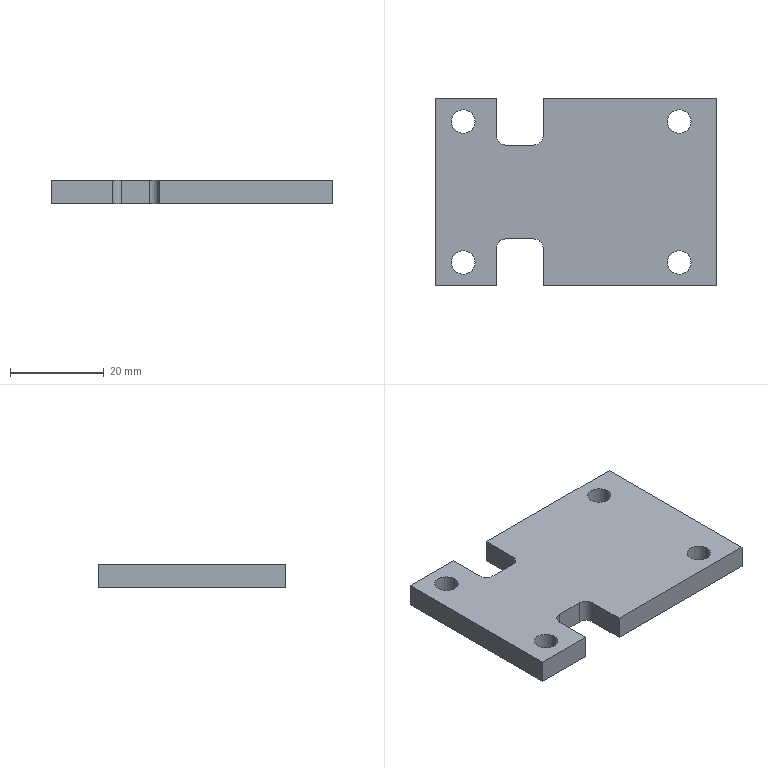Part | NX | 1 solid | 26 faces | box 60 x 40 x 5 mm | volume 10624 mm3 | plane 14 | cylinder 12 | commonest cylinder face diameters 5 x8 4 x4
STEP:
#1=CARTESIAN_POINT('',(-15.,-10.,-2.5));
#2=VERTEX_POINT('',#1);
#3=CARTESIAN_POINT('',(-9.,-10.,-2.5));
#4=VERTEX_POINT('',#3);
#5=CARTESIAN_POINT('',(0.,-10.,-2.5));
#6=DIRECTION('',(1.,0.,0.));
#7=VECTOR('',#6,1000.);
#8=LINE('',#5,#7);
#9=EDGE_CURVE('',#2,#4,#8,.T.);
#10=ORIENTED_EDGE('',*,*,#9,.F.);
#11=CARTESIAN_POINT('',(-17.,-12.,-2.5));
#12=VERTEX_POINT('',#11);
#13=CARTESIAN_POINT('',(-15.,-12.,-2.5));
#14=DIRECTION('',(0.,0.,-1.));
#15=DIRECTION('',(-1.,0.,0.));
#16=AXIS2_PLACEMENT_3D('',#13,#14,#15);
#17=CIRCLE('',#16,2.);
#18=EDGE_CURVE('',#12,#2,#17,.T.);
#19=ORIENTED_EDGE('',*,*,#18,.F.);
#20=CARTESIAN_POINT('',(-17.,-20.,-2.5));
#21=VERTEX_POINT('',#20);
#22=CARTESIAN_POINT('',(-17.,0.,-2.5));
#23=DIRECTION('',(0.,1.,0.));
#24=VECTOR('',#23,1000.);
#25=LINE('',#22,#24);
#26=EDGE_CURVE('',#21,#12,#25,.T.);
#27=ORIENTED_EDGE('',*,*,#26,.F.);
#28=CARTESIAN_POINT('',(-30.,-20.,-2.5));
#29=VERTEX_POINT('',#28);
#30=CARTESIAN_POINT('',(0.,-20.,-2.5));
#31=DIRECTION('',(-1.,0.,0.));
#32=VECTOR('',#31,1000.);
#33=LINE('',#30,#32);
#34=EDGE_CURVE('',#21,#29,#33,.T.);
#35=ORIENTED_EDGE('',*,*,#34,.T.);
#36=CARTESIAN_POINT('',(-30.,20.,-2.5));
#37=VERTEX_POINT('',#36);
#38=CARTESIAN_POINT('',(-30.,0.,-2.5));
#39=DIRECTION('',(0.,1.,0.));
#40=VECTOR('',#39,1000.);
#41=LINE('',#38,#40);
#42=EDGE_CURVE('',#29,#37,#41,.T.);
#43=ORIENTED_EDGE('',*,*,#42,.T.);
#44=CARTESIAN_POINT('',(-17.,20.,-2.5));
#45=VERTEX_POINT('',#44);
#46=CARTESIAN_POINT('',(0.,20.,-2.5));
#47=DIRECTION('',(1.,0.,0.));
#48=VECTOR('',#47,1000.);
#49=LINE('',#46,#48);
#50=EDGE_CURVE('',#37,#45,#49,.T.);
#51=ORIENTED_EDGE('',*,*,#50,.T.);
#52=CARTESIAN_POINT('',(-17.,12.,-2.5));
#53=VERTEX_POINT('',#52);
#54=CARTESIAN_POINT('',(-17.,0.,-2.5));
#55=DIRECTION('',(0.,1.,0.));
#56=VECTOR('',#55,1000.);
#57=LINE('',#54,#56);
#58=EDGE_CURVE('',#53,#45,#57,.T.);
#59=ORIENTED_EDGE('',*,*,#58,.F.);
#60=CARTESIAN_POINT('',(-15.,10.,-2.5));
#61=VERTEX_POINT('',#60);
#62=CARTESIAN_POINT('',(-15.,12.,-2.5));
#63=DIRECTION('',(0.,0.,-1.));
#64=DIRECTION('',(0.,-1.,0.));
#65=AXIS2_PLACEMENT_3D('',#62,#63,#64);
#66=CIRCLE('',#65,2.);
#67=EDGE_CURVE('',#61,#53,#66,.T.);
#68=ORIENTED_EDGE('',*,*,#67,.F.);
#69=CARTESIAN_POINT('',(-9.,10.,-2.5));
#70=VERTEX_POINT('',#69);
#71=CARTESIAN_POINT('',(0.,10.,-2.5));
#72=DIRECTION('',(-1.,0.,0.));
#73=VECTOR('',#72,1000.);
#74=LINE('',#71,#73);
#75=EDGE_CURVE('',#70,#61,#74,.T.);
#76=ORIENTED_EDGE('',*,*,#75,.F.);
#77=CARTESIAN_POINT('',(-7.,12.,-2.5));
#78=VERTEX_POINT('',#77);
#79=CARTESIAN_POINT('',(-9.,12.,-2.5));
#80=DIRECTION('',(0.,0.,-1.));
#81=DIRECTION('',(1.,0.,0.));
#82=AXIS2_PLACEMENT_3D('',#79,#80,#81);
#83=CIRCLE('',#82,2.);
#84=EDGE_CURVE('',#78,#70,#83,.T.);
#85=ORIENTED_EDGE('',*,*,#84,.F.);
#86=CARTESIAN_POINT('',(-7.,20.,-2.5));
#87=VERTEX_POINT('',#86);
#88=CARTESIAN_POINT('',(-7.,0.,-2.5));
#89=DIRECTION('',(0.,-1.,0.));
#90=VECTOR('',#89,1000.);
#91=LINE('',#88,#90);
#92=EDGE_CURVE('',#87,#78,#91,.T.);
#93=ORIENTED_EDGE('',*,*,#92,.F.);
#94=CARTESIAN_POINT('',(30.,20.,-2.5));
#95=VERTEX_POINT('',#94);
#96=CARTESIAN_POINT('',(0.,20.,-2.5));
#97=DIRECTION('',(1.,0.,0.));
#98=VECTOR('',#97,1000.);
#99=LINE('',#96,#98);
#100=EDGE_CURVE('',#87,#95,#99,.T.);
#101=ORIENTED_EDGE('',*,*,#100,.T.);
#102=CARTESIAN_POINT('',(30.,-20.,-2.5));
#103=VERTEX_POINT('',#102);
#104=CARTESIAN_POINT('',(30.,0.,-2.5));
#105=DIRECTION('',(0.,-1.,0.));
#106=VECTOR('',#105,1000.);
#107=LINE('',#104,#106);
#108=EDGE_CURVE('',#95,#103,#107,.T.);
#109=ORIENTED_EDGE('',*,*,#108,.T.);
#110=CARTESIAN_POINT('',(-7.,-20.,-2.5));
#111=VERTEX_POINT('',#110);
#112=CARTESIAN_POINT('',(0.,-20.,-2.5));
#113=DIRECTION('',(-1.,0.,0.));
#114=VECTOR('',#113,1000.);
#115=LINE('',#112,#114);
#116=EDGE_CURVE('',#103,#111,#115,.T.);
#117=ORIENTED_EDGE('',*,*,#116,.T.);
#118=CARTESIAN_POINT('',(-7.,-12.,-2.5));
#119=VERTEX_POINT('',#118);
#120=CARTESIAN_POINT('',(-7.,0.,-2.5));
#121=DIRECTION('',(0.,-1.,0.));
#122=VECTOR('',#121,1000.);
#123=LINE('',#120,#122);
#124=EDGE_CURVE('',#119,#111,#123,.T.);
#125=ORIENTED_EDGE('',*,*,#124,.F.);
#126=CARTESIAN_POINT('',(-9.,-12.,-2.5));
#127=DIRECTION('',(0.,0.,-1.));
#128=DIRECTION('',(0.,1.,0.));
#129=AXIS2_PLACEMENT_3D('',#126,#127,#128);
#130=CIRCLE('',#129,2.);
#131=EDGE_CURVE('',#4,#119,#130,.T.);
#132=ORIENTED_EDGE('',*,*,#131,.F.);
#133=EDGE_LOOP('',(#10,#19,#27,#35,#43,#51,#59,#68,#76,#85,#93,#101,#109,#117,#125,#132));
#134=FACE_BOUND('',#133,.T.);
#135=CARTESIAN_POINT('',(-21.5,-15.,-2.5));
#136=VERTEX_POINT('',#135);
#137=CARTESIAN_POINT('',(-26.5,-15.,-2.5));
#138=VERTEX_POINT('',#137);
#139=CARTESIAN_POINT('',(-24.,-15.,-2.5));
#140=DIRECTION('',(0.,0.,1.));
#141=DIRECTION('',(1.,0.,0.));
#142=AXIS2_PLACEMENT_3D('',#139,#140,#141);
#143=CIRCLE('',#142,2.5);
#144=EDGE_CURVE('',#136,#138,#143,.T.);
#145=ORIENTED_EDGE('',*,*,#144,.T.);
#146=CARTESIAN_POINT('',(-24.,-15.,-2.5));
#147=DIRECTION('',(0.,0.,1.));
#148=DIRECTION('',(1.,0.,0.));
#149=AXIS2_PLACEMENT_3D('',#146,#147,#148);
#150=CIRCLE('',#149,2.5);
#151=EDGE_CURVE('',#138,#136,#150,.T.);
#152=ORIENTED_EDGE('',*,*,#151,.T.);
#153=EDGE_LOOP('',(#145,#152));
#154=FACE_BOUND('',#153,.T.);
#155=CARTESIAN_POINT('',(-21.5,15.,-2.5));
#156=VERTEX_POINT('',#155);
#157=CARTESIAN_POINT('',(-26.5,15.,-2.5));
#158=VERTEX_POINT('',#157);
#159=CARTESIAN_POINT('',(-24.,15.,-2.5));
#160=DIRECTION('',(0.,0.,1.));
#161=DIRECTION('',(1.,0.,0.));
#162=AXIS2_PLACEMENT_3D('',#159,#160,#161);
#163=CIRCLE('',#162,2.5);
#164=EDGE_CURVE('',#156,#158,#163,.T.);
#165=ORIENTED_EDGE('',*,*,#164,.T.);
#166=CARTESIAN_POINT('',(-24.,15.,-2.5));
#167=DIRECTION('',(0.,0.,1.));
#168=DIRECTION('',(1.,0.,0.));
#169=AXIS2_PLACEMENT_3D('',#166,#167,#168);
#170=CIRCLE('',#169,2.5);
#171=EDGE_CURVE('',#158,#156,#170,.T.);
#172=ORIENTED_EDGE('',*,*,#171,.T.);
#173=EDGE_LOOP('',(#165,#172));
#174=FACE_BOUND('',#173,.T.);
#175=CARTESIAN_POINT('',(19.5,15.,-2.5));
#176=VERTEX_POINT('',#175);
#177=CARTESIAN_POINT('',(24.5,15.,-2.5));
#178=VERTEX_POINT('',#177);
#179=CARTESIAN_POINT('',(22.,15.,-2.5));
#180=DIRECTION('',(0.,0.,1.));
#181=DIRECTION('',(1.,0.,0.));
#182=AXIS2_PLACEMENT_3D('',#179,#180,#181);
#183=CIRCLE('',#182,2.5);
#184=EDGE_CURVE('',#176,#178,#183,.T.);
#185=ORIENTED_EDGE('',*,*,#184,.T.);
#186=CARTESIAN_POINT('',(22.,15.,-2.5));
#187=DIRECTION('',(0.,0.,1.));
#188=DIRECTION('',(1.,0.,0.));
#189=AXIS2_PLACEMENT_3D('',#186,#187,#188);
#190=CIRCLE('',#189,2.5);
#191=EDGE_CURVE('',#178,#176,#190,.T.);
#192=ORIENTED_EDGE('',*,*,#191,.T.);
#193=EDGE_LOOP('',(#185,#192));
#194=FACE_BOUND('',#193,.T.);
#195=CARTESIAN_POINT('',(19.5,-15.,-2.5));
#196=VERTEX_POINT('',#195);
#197=CARTESIAN_POINT('',(24.5,-15.,-2.5));
#198=VERTEX_POINT('',#197);
#199=CARTESIAN_POINT('',(22.,-15.,-2.5));
#200=DIRECTION('',(0.,0.,1.));
#201=DIRECTION('',(1.,0.,0.));
#202=AXIS2_PLACEMENT_3D('',#199,#200,#201);
#203=CIRCLE('',#202,2.5);
#204=EDGE_CURVE('',#196,#198,#203,.T.);
#205=ORIENTED_EDGE('',*,*,#204,.T.);
#206=CARTESIAN_POINT('',(22.,-15.,-2.5));
#207=DIRECTION('',(0.,0.,1.));
#208=DIRECTION('',(1.,0.,0.));
#209=AXIS2_PLACEMENT_3D('',#206,#207,#208);
#210=CIRCLE('',#209,2.5);
#211=EDGE_CURVE('',#198,#196,#210,.T.);
#212=ORIENTED_EDGE('',*,*,#211,.T.);
#213=EDGE_LOOP('',(#205,#212));
#214=FACE_BOUND('',#213,.T.);
#215=CARTESIAN_POINT('',(0.,0.,-2.5));
#216=DIRECTION('',(0.,0.,1.));
#217=DIRECTION('',(1.,0.,0.));
#218=AXIS2_PLACEMENT_3D('',#215,#216,#217);
#219=PLANE('',#218);
#220=ADVANCED_FACE('',(#134,#154,#174,#194,#214),#219,.F.);
#221=CARTESIAN_POINT('',(-15.,-10.,2.5));
#222=VERTEX_POINT('',#221);
#223=CARTESIAN_POINT('',(-15.,-10.,2.5));
#224=DIRECTION('',(0.,0.,-1.));
#225=VECTOR('',#224,1000.);
#226=LINE('',#223,#225);
#227=EDGE_CURVE('',#222,#2,#226,.T.);
#228=ORIENTED_EDGE('',*,*,#227,.T.);
#229=ORIENTED_EDGE('',*,*,#9,.T.);
#230=CARTESIAN_POINT('',(-9.,-10.,2.5));
#231=VERTEX_POINT('',#230);
#232=CARTESIAN_POINT('',(-9.,-10.,2.624));
#233=DIRECTION('',(0.,0.,-1.));
#234=VECTOR('',#233,1000.);
#235=LINE('',#232,#234);
#236=EDGE_CURVE('',#231,#4,#235,.T.);
#237=ORIENTED_EDGE('',*,*,#236,.F.);
#238=CARTESIAN_POINT('',(0.,-10.,2.5));
#239=DIRECTION('',(1.,0.,0.));
#240=VECTOR('',#239,1000.);
#241=LINE('',#238,#240);
#242=EDGE_CURVE('',#222,#231,#241,.T.);
#243=ORIENTED_EDGE('',*,*,#242,.F.);
#244=EDGE_LOOP('',(#228,#229,#237,#243));
#245=FACE_BOUND('',#244,.T.);
#246=CARTESIAN_POINT('',(-7.,-10.,2.5));
#247=DIRECTION('',(0.,1.,0.));
#248=DIRECTION('',(1.,0.,0.));
#249=AXIS2_PLACEMENT_3D('',#246,#247,#248);
#250=PLANE('',#249);
#251=ADVANCED_FACE('',(#245),#250,.F.);
#252=CARTESIAN_POINT('',(-17.,-12.,2.5));
#253=VERTEX_POINT('',#252);
#254=CARTESIAN_POINT('',(-17.,-12.,2.624));
#255=DIRECTION('',(0.,0.,-1.));
#256=VECTOR('',#255,1000.);
#257=LINE('',#254,#256);
#258=EDGE_CURVE('',#253,#12,#257,.T.);
#259=ORIENTED_EDGE('',*,*,#258,.T.);
#260=ORIENTED_EDGE('',*,*,#18,.T.);
#261=ORIENTED_EDGE('',*,*,#227,.F.);
#262=CARTESIAN_POINT('',(-15.,-12.,2.5));
#263=DIRECTION('',(0.,0.,-1.));
#264=DIRECTION('',(-1.,0.,0.));
#265=AXIS2_PLACEMENT_3D('',#262,#263,#264);
#266=CIRCLE('',#265,2.);
#267=EDGE_CURVE('',#253,#222,#266,.T.);
#268=ORIENTED_EDGE('',*,*,#267,.F.);
#269=EDGE_LOOP('',(#259,#260,#261,#268));
#270=FACE_BOUND('',#269,.T.);
#271=CARTESIAN_POINT('',(-15.,-12.,2.624));
#272=DIRECTION('',(0.,0.,-1.));
#273=DIRECTION('',(-1.,0.,0.));
#274=AXIS2_PLACEMENT_3D('',#271,#272,#273);
#275=CYLINDRICAL_SURFACE('',#274,2.);
#276=ADVANCED_FACE('',(#270),#275,.F.);
#277=ORIENTED_EDGE('',*,*,#258,.F.);
#278=CARTESIAN_POINT('',(-17.,-20.,2.5));
#279=VERTEX_POINT('',#278);
#280=CARTESIAN_POINT('',(-17.,0.,2.5));
#281=DIRECTION('',(0.,1.,0.));
#282=VECTOR('',#281,1000.);
#283=LINE('',#280,#282);
#284=EDGE_CURVE('',#279,#253,#283,.T.);
#285=ORIENTED_EDGE('',*,*,#284,.F.);
#286=CARTESIAN_POINT('',(-17.,-20.,0.));
#287=DIRECTION('',(0.,0.,1.));
#288=VECTOR('',#287,1000.);
#289=LINE('',#286,#288);
#290=EDGE_CURVE('',#21,#279,#289,.T.);
#291=ORIENTED_EDGE('',*,*,#290,.F.);
#292=ORIENTED_EDGE('',*,*,#26,.T.);
#293=EDGE_LOOP('',(#277,#285,#291,#292));
#294=FACE_BOUND('',#293,.T.);
#295=CARTESIAN_POINT('',(-17.,-10.,2.5));
#296=DIRECTION('',(-1.,0.,0.));
#297=DIRECTION('',(0.,0.,1.));
#298=AXIS2_PLACEMENT_3D('',#295,#296,#297);
#299=PLANE('',#298);
#300=ADVANCED_FACE('',(#294),#299,.F.);
#301=ORIENTED_EDGE('',*,*,#290,.T.);
#302=CARTESIAN_POINT('',(-30.,-20.,2.5));
#303=VERTEX_POINT('',#302);
#304=CARTESIAN_POINT('',(0.,-20.,2.5));
#305=DIRECTION('',(-1.,0.,0.));
#306=VECTOR('',#305,1000.);
#307=LINE('',#304,#306);
#308=EDGE_CURVE('',#279,#303,#307,.T.);
#309=ORIENTED_EDGE('',*,*,#308,.T.);
#310=CARTESIAN_POINT('',(-30.,-20.,0.));
#311=DIRECTION('',(0.,0.,1.));
#312=VECTOR('',#311,1000.);
#313=LINE('',#310,#312);
#314=EDGE_CURVE('',#29,#303,#313,.T.);
#315=ORIENTED_EDGE('',*,*,#314,.F.);
#316=ORIENTED_EDGE('',*,*,#34,.F.);
#317=EDGE_LOOP('',(#301,#309,#315,#316));
#318=FACE_BOUND('',#317,.T.);
#319=CARTESIAN_POINT('',(-30.,-20.,-2.5));
#320=DIRECTION('',(0.,-1.,0.));
#321=DIRECTION('',(0.,0.,-1.));
#322=AXIS2_PLACEMENT_3D('',#319,#320,#321);
#323=PLANE('',#322);
#324=ADVANCED_FACE('',(#318),#323,.T.);
#325=ORIENTED_EDGE('',*,*,#42,.F.);
#326=ORIENTED_EDGE('',*,*,#314,.T.);
#327=CARTESIAN_POINT('',(-30.,20.,2.5));
#328=VERTEX_POINT('',#327);
#329=CARTESIAN_POINT('',(-30.,0.,2.5));
#330=DIRECTION('',(0.,1.,0.));
#331=VECTOR('',#330,1000.);
#332=LINE('',#329,#331);
#333=EDGE_CURVE('',#303,#328,#332,.T.);
#334=ORIENTED_EDGE('',*,*,#333,.T.);
#335=CARTESIAN_POINT('',(-30.,20.,0.));
#336=DIRECTION('',(0.,0.,-1.));
#337=VECTOR('',#336,1000.);
#338=LINE('',#335,#337);
#339=EDGE_CURVE('',#328,#37,#338,.T.);
#340=ORIENTED_EDGE('',*,*,#339,.T.);
#341=EDGE_LOOP('',(#325,#326,#334,#340));
#342=FACE_BOUND('',#341,.T.);
#343=CARTESIAN_POINT('',(-30.,20.,-2.5));
#344=DIRECTION('',(-1.,0.,0.));
#345=DIRECTION('',(0.,0.,1.));
#346=AXIS2_PLACEMENT_3D('',#343,#344,#345);
#347=PLANE('',#346);
#348=ADVANCED_FACE('',(#342),#347,.T.);
#349=CARTESIAN_POINT('',(-17.,20.,2.5));
#350=VERTEX_POINT('',#349);
#351=CARTESIAN_POINT('',(-17.,20.,0.));
#352=DIRECTION('',(0.,0.,1.));
#353=VECTOR('',#352,1000.);
#354=LINE('',#351,#353);
#355=EDGE_CURVE('',#45,#350,#354,.T.);
#356=ORIENTED_EDGE('',*,*,#355,.F.);
#357=ORIENTED_EDGE('',*,*,#50,.F.);
#358=ORIENTED_EDGE('',*,*,#339,.F.);
#359=CARTESIAN_POINT('',(0.,20.,2.5));
#360=DIRECTION('',(1.,0.,0.));
#361=VECTOR('',#360,1000.);
#362=LINE('',#359,#361);
#363=EDGE_CURVE('',#328,#350,#362,.T.);
#364=ORIENTED_EDGE('',*,*,#363,.T.);
#365=EDGE_LOOP('',(#356,#357,#358,#364));
#366=FACE_BOUND('',#365,.T.);
#367=CARTESIAN_POINT('',(30.,20.,-2.5));
#368=DIRECTION('',(0.,1.,0.));
#369=DIRECTION('',(1.,0.,0.));
#370=AXIS2_PLACEMENT_3D('',#367,#368,#369);
#371=PLANE('',#370);
#372=ADVANCED_FACE('',(#366),#371,.T.);
#373=CARTESIAN_POINT('',(-17.,12.,2.5));
#374=VERTEX_POINT('',#373);
#375=CARTESIAN_POINT('',(-17.,12.,2.5));
#376=DIRECTION('',(0.,0.,-1.));
#377=VECTOR('',#376,1000.);
#378=LINE('',#375,#377);
#379=EDGE_CURVE('',#374,#53,#378,.T.);
#380=ORIENTED_EDGE('',*,*,#379,.T.);
#381=ORIENTED_EDGE('',*,*,#58,.T.);
#382=ORIENTED_EDGE('',*,*,#355,.T.);
#383=CARTESIAN_POINT('',(-17.,0.,2.5));
#384=DIRECTION('',(0.,-1.,0.));
#385=VECTOR('',#384,1000.);
#386=LINE('',#383,#385);
#387=EDGE_CURVE('',#350,#374,#386,.T.);
#388=ORIENTED_EDGE('',*,*,#387,.T.);
#389=EDGE_LOOP('',(#380,#381,#382,#388));
#390=FACE_BOUND('',#389,.T.);
#391=CARTESIAN_POINT('',(-17.,20.,2.5));
#392=DIRECTION('',(-1.,0.,0.));
#393=DIRECTION('',(0.,0.,1.));
#394=AXIS2_PLACEMENT_3D('',#391,#392,#393);
#395=PLANE('',#394);
#396=ADVANCED_FACE('',(#390),#395,.F.);
#397=CARTESIAN_POINT('',(-15.,10.,2.5));
#398=VERTEX_POINT('',#397);
#399=CARTESIAN_POINT('',(-15.,10.,2.624));
#400=DIRECTION('',(0.,0.,-1.));
#401=VECTOR('',#400,1000.);
#402=LINE('',#399,#401);
#403=EDGE_CURVE('',#398,#61,#402,.T.);
#404=ORIENTED_EDGE('',*,*,#403,.T.);
#405=ORIENTED_EDGE('',*,*,#67,.T.);
#406=ORIENTED_EDGE('',*,*,#379,.F.);
#407=CARTESIAN_POINT('',(-15.,12.,2.5));
#408=DIRECTION('',(0.,0.,-1.));
#409=DIRECTION('',(0.,-1.,0.));
#410=AXIS2_PLACEMENT_3D('',#407,#408,#409);
#411=CIRCLE('',#410,2.);
#412=EDGE_CURVE('',#398,#374,#411,.T.);
#413=ORIENTED_EDGE('',*,*,#412,.F.);
#414=EDGE_LOOP('',(#404,#405,#406,#413));
#415=FACE_BOUND('',#414,.T.);
#416=CARTESIAN_POINT('',(-15.,12.,2.624));
#417=DIRECTION('',(0.,0.,-1.));
#418=DIRECTION('',(0.,-1.,0.));
#419=AXIS2_PLACEMENT_3D('',#416,#417,#418);
#420=CYLINDRICAL_SURFACE('',#419,2.);
#421=ADVANCED_FACE('',(#415),#420,.F.);
#422=CARTESIAN_POINT('',(-9.,10.,2.5));
#423=VERTEX_POINT('',#422);
#424=CARTESIAN_POINT('',(-9.,10.,2.5));
#425=DIRECTION('',(0.,0.,-1.));
#426=VECTOR('',#425,1000.);
#427=LINE('',#424,#426);
#428=EDGE_CURVE('',#423,#70,#427,.T.);
#429=ORIENTED_EDGE('',*,*,#428,.T.);
#430=ORIENTED_EDGE('',*,*,#75,.T.);
#431=ORIENTED_EDGE('',*,*,#403,.F.);
#432=CARTESIAN_POINT('',(0.,10.,2.5));
#433=DIRECTION('',(-1.,0.,0.));
#434=VECTOR('',#433,1000.);
#435=LINE('',#432,#434);
#436=EDGE_CURVE('',#423,#398,#435,.T.);
#437=ORIENTED_EDGE('',*,*,#436,.F.);
#438=EDGE_LOOP('',(#429,#430,#431,#437));
#439=FACE_BOUND('',#438,.T.);
#440=CARTESIAN_POINT('',(-17.,10.,2.5));
#441=DIRECTION('',(0.,-1.,0.));
#442=DIRECTION('',(0.,0.,-1.));
#443=AXIS2_PLACEMENT_3D('',#440,#441,#442);
#444=PLANE('',#443);
#445=ADVANCED_FACE('',(#439),#444,.F.);
#446=CARTESIAN_POINT('',(-7.,12.,2.5));
#447=VERTEX_POINT('',#446);
#448=CARTESIAN_POINT('',(-7.,12.,2.624));
#449=DIRECTION('',(0.,0.,-1.));
#450=VECTOR('',#449,1000.);
#451=LINE('',#448,#450);
#452=EDGE_CURVE('',#447,#78,#451,.T.);
#453=ORIENTED_EDGE('',*,*,#452,.T.);
#454=ORIENTED_EDGE('',*,*,#84,.T.);
#455=ORIENTED_EDGE('',*,*,#428,.F.);
#456=CARTESIAN_POINT('',(-9.,12.,2.5));
#457=DIRECTION('',(0.,0.,-1.));
#458=DIRECTION('',(1.,0.,0.));
#459=AXIS2_PLACEMENT_3D('',#456,#457,#458);
#460=CIRCLE('',#459,2.);
#461=EDGE_CURVE('',#447,#423,#460,.T.);
#462=ORIENTED_EDGE('',*,*,#461,.F.);
#463=EDGE_LOOP('',(#453,#454,#455,#462));
#464=FACE_BOUND('',#463,.T.);
#465=CARTESIAN_POINT('',(-9.,12.,2.624));
#466=DIRECTION('',(0.,0.,-1.));
#467=DIRECTION('',(1.,0.,0.));
#468=AXIS2_PLACEMENT_3D('',#465,#466,#467);
#469=CYLINDRICAL_SURFACE('',#468,2.);
#470=ADVANCED_FACE('',(#464),#469,.F.);
#471=ORIENTED_EDGE('',*,*,#452,.F.);
#472=CARTESIAN_POINT('',(-7.,20.,2.5));
#473=VERTEX_POINT('',#472);
#474=CARTESIAN_POINT('',(-7.,0.,2.5));
#475=DIRECTION('',(0.,-1.,0.));
#476=VECTOR('',#475,1000.);
#477=LINE('',#474,#476);
#478=EDGE_CURVE('',#473,#447,#477,.T.);
#479=ORIENTED_EDGE('',*,*,#478,.F.);
#480=CARTESIAN_POINT('',(-7.,20.,0.));
#481=DIRECTION('',(0.,0.,1.));
#482=VECTOR('',#481,1000.);
#483=LINE('',#480,#482);
#484=EDGE_CURVE('',#87,#473,#483,.T.);
#485=ORIENTED_EDGE('',*,*,#484,.F.);
#486=ORIENTED_EDGE('',*,*,#92,.T.);
#487=EDGE_LOOP('',(#471,#479,#485,#486));
#488=FACE_BOUND('',#487,.T.);
#489=CARTESIAN_POINT('',(-7.,10.,2.5));
#490=DIRECTION('',(1.,0.,0.));
#491=DIRECTION('',(0.,1.,0.));
#492=AXIS2_PLACEMENT_3D('',#489,#490,#491);
#493=PLANE('',#492);
#494=ADVANCED_FACE('',(#488),#493,.F.);
#495=ORIENTED_EDGE('',*,*,#484,.T.);
#496=CARTESIAN_POINT('',(30.,20.,2.5));
#497=VERTEX_POINT('',#496);
#498=CARTESIAN_POINT('',(0.,20.,2.5));
#499=DIRECTION('',(1.,0.,0.));
#500=VECTOR('',#499,1000.);
#501=LINE('',#498,#500);
#502=EDGE_CURVE('',#473,#497,#501,.T.);
#503=ORIENTED_EDGE('',*,*,#502,.T.);
#504=CARTESIAN_POINT('',(30.,20.,0.));
#505=DIRECTION('',(0.,0.,1.));
#506=VECTOR('',#505,1000.);
#507=LINE('',#504,#506);
#508=EDGE_CURVE('',#95,#497,#507,.T.);
#509=ORIENTED_EDGE('',*,*,#508,.F.);
#510=ORIENTED_EDGE('',*,*,#100,.F.);
#511=EDGE_LOOP('',(#495,#503,#509,#510));
#512=FACE_BOUND('',#511,.T.);
#513=CARTESIAN_POINT('',(30.,20.,-2.5));
#514=DIRECTION('',(0.,1.,0.));
#515=DIRECTION('',(1.,0.,0.));
#516=AXIS2_PLACEMENT_3D('',#513,#514,#515);
#517=PLANE('',#516);
#518=ADVANCED_FACE('',(#512),#517,.T.);
#519=ORIENTED_EDGE('',*,*,#108,.F.);
#520=ORIENTED_EDGE('',*,*,#508,.T.);
#521=CARTESIAN_POINT('',(30.,-20.,2.5));
#522=VERTEX_POINT('',#521);
#523=CARTESIAN_POINT('',(30.,0.,2.5));
#524=DIRECTION('',(0.,-1.,0.));
#525=VECTOR('',#524,1000.);
#526=LINE('',#523,#525);
#527=EDGE_CURVE('',#497,#522,#526,.T.);
#528=ORIENTED_EDGE('',*,*,#527,.T.);
#529=CARTESIAN_POINT('',(30.,-20.,0.));
#530=DIRECTION('',(0.,0.,-1.));
#531=VECTOR('',#530,1000.);
#532=LINE('',#529,#531);
#533=EDGE_CURVE('',#522,#103,#532,.T.);
#534=ORIENTED_EDGE('',*,*,#533,.T.);
#535=EDGE_LOOP('',(#519,#520,#528,#534));
#536=FACE_BOUND('',#535,.T.);
#537=CARTESIAN_POINT('',(30.,-20.,-2.5));
#538=DIRECTION('',(1.,0.,0.));
#539=DIRECTION('',(0.,1.,0.));
#540=AXIS2_PLACEMENT_3D('',#537,#538,#539);
#541=PLANE('',#540);
#542=ADVANCED_FACE('',(#536),#541,.T.);
#543=CARTESIAN_POINT('',(-7.,-20.,2.5));
#544=VERTEX_POINT('',#543);
#545=CARTESIAN_POINT('',(-7.,-20.,0.));
#546=DIRECTION('',(0.,0.,1.));
#547=VECTOR('',#546,1000.);
#548=LINE('',#545,#547);
#549=EDGE_CURVE('',#111,#544,#548,.T.);
#550=ORIENTED_EDGE('',*,*,#549,.F.);
#551=ORIENTED_EDGE('',*,*,#116,.F.);
#552=ORIENTED_EDGE('',*,*,#533,.F.);
#553=CARTESIAN_POINT('',(0.,-20.,2.5));
#554=DIRECTION('',(-1.,0.,0.));
#555=VECTOR('',#554,1000.);
#556=LINE('',#553,#555);
#557=EDGE_CURVE('',#522,#544,#556,.T.);
#558=ORIENTED_EDGE('',*,*,#557,.T.);
#559=EDGE_LOOP('',(#550,#551,#552,#558));
#560=FACE_BOUND('',#559,.T.);
#561=CARTESIAN_POINT('',(-30.,-20.,-2.5));
#562=DIRECTION('',(0.,-1.,0.));
#563=DIRECTION('',(0.,0.,-1.));
#564=AXIS2_PLACEMENT_3D('',#561,#562,#563);
#565=PLANE('',#564);
#566=ADVANCED_FACE('',(#560),#565,.T.);
#567=CARTESIAN_POINT('',(-7.,-12.,2.5));
#568=VERTEX_POINT('',#567);
#569=CARTESIAN_POINT('',(-7.,-12.,2.5));
#570=DIRECTION('',(0.,0.,-1.));
#571=VECTOR('',#570,1000.);
#572=LINE('',#569,#571);
#573=EDGE_CURVE('',#568,#119,#572,.T.);
#574=ORIENTED_EDGE('',*,*,#573,.T.);
#575=ORIENTED_EDGE('',*,*,#124,.T.);
#576=ORIENTED_EDGE('',*,*,#549,.T.);
#577=CARTESIAN_POINT('',(-7.,0.,2.5));
#578=DIRECTION('',(0.,-1.,0.));
#579=VECTOR('',#578,1000.);
#580=LINE('',#577,#579);
#581=EDGE_CURVE('',#568,#544,#580,.T.);
#582=ORIENTED_EDGE('',*,*,#581,.F.);
#583=EDGE_LOOP('',(#574,#575,#576,#582));
#584=FACE_BOUND('',#583,.T.);
#585=CARTESIAN_POINT('',(-7.,-20.,2.5));
#586=DIRECTION('',(1.,0.,0.));
#587=DIRECTION('',(0.,1.,0.));
#588=AXIS2_PLACEMENT_3D('',#585,#586,#587);
#589=PLANE('',#588);
#590=ADVANCED_FACE('',(#584),#589,.F.);
#591=ORIENTED_EDGE('',*,*,#236,.T.);
#592=ORIENTED_EDGE('',*,*,#131,.T.);
#593=ORIENTED_EDGE('',*,*,#573,.F.);
#594=CARTESIAN_POINT('',(-9.,-12.,2.5));
#595=DIRECTION('',(0.,0.,-1.));
#596=DIRECTION('',(0.,1.,0.));
#597=AXIS2_PLACEMENT_3D('',#594,#595,#596);
#598=CIRCLE('',#597,2.);
#599=EDGE_CURVE('',#231,#568,#598,.T.);
#600=ORIENTED_EDGE('',*,*,#599,.F.);
#601=EDGE_LOOP('',(#591,#592,#593,#600));
#602=FACE_BOUND('',#601,.T.);
#603=CARTESIAN_POINT('',(-9.,-12.,2.624));
#604=DIRECTION('',(0.,0.,-1.));
#605=DIRECTION('',(0.,1.,0.));
#606=AXIS2_PLACEMENT_3D('',#603,#604,#605);
#607=CYLINDRICAL_SURFACE('',#606,2.);
#608=ADVANCED_FACE('',(#602),#607,.F.);
#609=ORIENTED_EDGE('',*,*,#581,.T.);
#610=ORIENTED_EDGE('',*,*,#557,.F.);
#611=ORIENTED_EDGE('',*,*,#527,.F.);
#612=ORIENTED_EDGE('',*,*,#502,.F.);
#613=ORIENTED_EDGE('',*,*,#478,.T.);
#614=ORIENTED_EDGE('',*,*,#461,.T.);
#615=ORIENTED_EDGE('',*,*,#436,.T.);
#616=ORIENTED_EDGE('',*,*,#412,.T.);
#617=ORIENTED_EDGE('',*,*,#387,.F.);
#618=ORIENTED_EDGE('',*,*,#363,.F.);
#619=ORIENTED_EDGE('',*,*,#333,.F.);
#620=ORIENTED_EDGE('',*,*,#308,.F.);
#621=ORIENTED_EDGE('',*,*,#284,.T.);
#622=ORIENTED_EDGE('',*,*,#267,.T.);
#623=ORIENTED_EDGE('',*,*,#242,.T.);
#624=ORIENTED_EDGE('',*,*,#599,.T.);
#625=EDGE_LOOP('',(#609,#610,#611,#612,#613,#614,#615,#616,#617,#618,#619,#620,#621,#622,#623,#624));
#626=FACE_BOUND('',#625,.T.);
#627=CARTESIAN_POINT('',(-26.5,-15.,2.5));
#628=VERTEX_POINT('',#627);
#629=CARTESIAN_POINT('',(-21.5,-15.,2.5));
#630=VERTEX_POINT('',#629);
#631=CARTESIAN_POINT('',(-24.,-15.,2.5));
#632=DIRECTION('',(0.,0.,1.));
#633=DIRECTION('',(1.,0.,0.));
#634=AXIS2_PLACEMENT_3D('',#631,#632,#633);
#635=CIRCLE('',#634,2.5);
#636=EDGE_CURVE('',#628,#630,#635,.T.);
#637=ORIENTED_EDGE('',*,*,#636,.F.);
#638=CARTESIAN_POINT('',(-24.,-15.,2.5));
#639=DIRECTION('',(0.,0.,1.));
#640=DIRECTION('',(1.,0.,0.));
#641=AXIS2_PLACEMENT_3D('',#638,#639,#640);
#642=CIRCLE('',#641,2.5);
#643=EDGE_CURVE('',#630,#628,#642,.T.);
#644=ORIENTED_EDGE('',*,*,#643,.F.);
#645=EDGE_LOOP('',(#637,#644));
#646=FACE_BOUND('',#645,.T.);
#647=CARTESIAN_POINT('',(-26.5,15.,2.5));
#648=VERTEX_POINT('',#647);
#649=CARTESIAN_POINT('',(-21.5,15.,2.5));
#650=VERTEX_POINT('',#649);
#651=CARTESIAN_POINT('',(-24.,15.,2.5));
#652=DIRECTION('',(0.,0.,1.));
#653=DIRECTION('',(1.,0.,0.));
#654=AXIS2_PLACEMENT_3D('',#651,#652,#653);
#655=CIRCLE('',#654,2.5);
#656=EDGE_CURVE('',#648,#650,#655,.T.);
#657=ORIENTED_EDGE('',*,*,#656,.F.);
#658=CARTESIAN_POINT('',(-24.,15.,2.5));
#659=DIRECTION('',(0.,0.,1.));
#660=DIRECTION('',(1.,0.,0.));
#661=AXIS2_PLACEMENT_3D('',#658,#659,#660);
#662=CIRCLE('',#661,2.5);
#663=EDGE_CURVE('',#650,#648,#662,.T.);
#664=ORIENTED_EDGE('',*,*,#663,.F.);
#665=EDGE_LOOP('',(#657,#664));
#666=FACE_BOUND('',#665,.T.);
#667=CARTESIAN_POINT('',(19.5,15.,2.5));
#668=VERTEX_POINT('',#667);
#669=CARTESIAN_POINT('',(24.5,15.,2.5));
#670=VERTEX_POINT('',#669);
#671=CARTESIAN_POINT('',(22.,15.,2.5));
#672=DIRECTION('',(0.,0.,1.));
#673=DIRECTION('',(1.,0.,0.));
#674=AXIS2_PLACEMENT_3D('',#671,#672,#673);
#675=CIRCLE('',#674,2.5);
#676=EDGE_CURVE('',#668,#670,#675,.T.);
#677=ORIENTED_EDGE('',*,*,#676,.F.);
#678=CARTESIAN_POINT('',(22.,15.,2.5));
#679=DIRECTION('',(0.,0.,1.));
#680=DIRECTION('',(1.,0.,0.));
#681=AXIS2_PLACEMENT_3D('',#678,#679,#680);
#682=CIRCLE('',#681,2.5);
#683=EDGE_CURVE('',#670,#668,#682,.T.);
#684=ORIENTED_EDGE('',*,*,#683,.F.);
#685=EDGE_LOOP('',(#677,#684));
#686=FACE_BOUND('',#685,.T.);
#687=CARTESIAN_POINT('',(24.5,-15.,2.5));
#688=VERTEX_POINT('',#687);
#689=CARTESIAN_POINT('',(19.5,-15.,2.5));
#690=VERTEX_POINT('',#689);
#691=CARTESIAN_POINT('',(22.,-15.,2.5));
#692=DIRECTION('',(0.,0.,1.));
#693=DIRECTION('',(1.,0.,0.));
#694=AXIS2_PLACEMENT_3D('',#691,#692,#693);
#695=CIRCLE('',#694,2.5);
#696=EDGE_CURVE('',#688,#690,#695,.T.);
#697=ORIENTED_EDGE('',*,*,#696,.F.);
#698=CARTESIAN_POINT('',(22.,-15.,2.5));
#699=DIRECTION('',(0.,0.,1.));
#700=DIRECTION('',(1.,0.,0.));
#701=AXIS2_PLACEMENT_3D('',#698,#699,#700);
#702=CIRCLE('',#701,2.5);
#703=EDGE_CURVE('',#690,#688,#702,.T.);
#704=ORIENTED_EDGE('',*,*,#703,.F.);
#705=EDGE_LOOP('',(#697,#704));
#706=FACE_BOUND('',#705,.T.);
#707=CARTESIAN_POINT('',(0.,0.,2.5));
#708=DIRECTION('',(0.,0.,1.));
#709=DIRECTION('',(1.,0.,0.));
#710=AXIS2_PLACEMENT_3D('',#707,#708,#709);
#711=PLANE('',#710);
#712=ADVANCED_FACE('',(#626,#646,#666,#686,#706),#711,.T.);
#713=ORIENTED_EDGE('',*,*,#636,.T.);
#714=CARTESIAN_POINT('',(-21.5,-15.,-2.5));
#715=DIRECTION('',(0.,0.,1.));
#716=VECTOR('',#715,1000.);
#717=LINE('',#714,#716);
#718=EDGE_CURVE('',#136,#630,#717,.T.);
#719=ORIENTED_EDGE('',*,*,#718,.F.);
#720=ORIENTED_EDGE('',*,*,#151,.F.);
#721=CARTESIAN_POINT('',(-26.5,-15.,-2.5));
#722=DIRECTION('',(0.,0.,1.));
#723=VECTOR('',#722,1000.);
#724=LINE('',#721,#723);
#725=EDGE_CURVE('',#138,#628,#724,.T.);
#726=ORIENTED_EDGE('',*,*,#725,.T.);
#727=EDGE_LOOP('',(#713,#719,#720,#726));
#728=FACE_BOUND('',#727,.T.);
#729=CARTESIAN_POINT('',(-24.,-15.,-2.5));
#730=DIRECTION('',(0.,0.,1.));
#731=DIRECTION('',(1.,0.,0.));
#732=AXIS2_PLACEMENT_3D('',#729,#730,#731);
#733=CYLINDRICAL_SURFACE('',#732,2.5);
#734=ADVANCED_FACE('',(#728),#733,.F.);
#735=ORIENTED_EDGE('',*,*,#164,.F.);
#736=CARTESIAN_POINT('',(-21.5,15.,-2.5));
#737=DIRECTION('',(0.,0.,1.));
#738=VECTOR('',#737,1000.);
#739=LINE('',#736,#738);
#740=EDGE_CURVE('',#156,#650,#739,.T.);
#741=ORIENTED_EDGE('',*,*,#740,.T.);
#742=ORIENTED_EDGE('',*,*,#663,.T.);
#743=CARTESIAN_POINT('',(-26.5,15.,-2.5));
#744=DIRECTION('',(0.,0.,1.));
#745=VECTOR('',#744,1000.);
#746=LINE('',#743,#745);
#747=EDGE_CURVE('',#158,#648,#746,.T.);
#748=ORIENTED_EDGE('',*,*,#747,.F.);
#749=EDGE_LOOP('',(#735,#741,#742,#748));
#750=FACE_BOUND('',#749,.T.);
#751=CARTESIAN_POINT('',(-24.,15.,-2.5));
#752=DIRECTION('',(0.,0.,1.));
#753=DIRECTION('',(1.,0.,0.));
#754=AXIS2_PLACEMENT_3D('',#751,#752,#753);
#755=CYLINDRICAL_SURFACE('',#754,2.5);
#756=ADVANCED_FACE('',(#750),#755,.F.);
#757=ORIENTED_EDGE('',*,*,#696,.T.);
#758=CARTESIAN_POINT('',(19.5,-15.,-2.5));
#759=DIRECTION('',(0.,0.,1.));
#760=VECTOR('',#759,1000.);
#761=LINE('',#758,#760);
#762=EDGE_CURVE('',#690,#196,#761,.F.);
#763=ORIENTED_EDGE('',*,*,#762,.T.);
#764=ORIENTED_EDGE('',*,*,#211,.F.);
#765=CARTESIAN_POINT('',(24.5,-15.,-2.5));
#766=DIRECTION('',(0.,0.,1.));
#767=VECTOR('',#766,1000.);
#768=LINE('',#765,#767);
#769=EDGE_CURVE('',#688,#198,#768,.F.);
#770=ORIENTED_EDGE('',*,*,#769,.F.);
#771=EDGE_LOOP('',(#757,#763,#764,#770));
#772=FACE_BOUND('',#771,.T.);
#773=CARTESIAN_POINT('',(22.,-15.,-2.5));
#774=DIRECTION('',(0.,0.,1.));
#775=DIRECTION('',(1.,0.,0.));
#776=AXIS2_PLACEMENT_3D('',#773,#774,#775);
#777=CYLINDRICAL_SURFACE('',#776,2.5);
#778=ADVANCED_FACE('',(#772),#777,.F.);
#779=ORIENTED_EDGE('',*,*,#184,.F.);
#780=CARTESIAN_POINT('',(19.5,15.,-2.5));
#781=DIRECTION('',(0.,0.,1.));
#782=VECTOR('',#781,1000.);
#783=LINE('',#780,#782);
#784=EDGE_CURVE('',#176,#668,#783,.T.);
#785=ORIENTED_EDGE('',*,*,#784,.T.);
#786=ORIENTED_EDGE('',*,*,#676,.T.);
#787=CARTESIAN_POINT('',(24.5,15.,-2.5));
#788=DIRECTION('',(0.,0.,1.));
#789=VECTOR('',#788,1000.);
#790=LINE('',#787,#789);
#791=EDGE_CURVE('',#178,#670,#790,.T.);
#792=ORIENTED_EDGE('',*,*,#791,.F.);
#793=EDGE_LOOP('',(#779,#785,#786,#792));
#794=FACE_BOUND('',#793,.T.);
#795=CARTESIAN_POINT('',(22.,15.,-2.5));
#796=DIRECTION('',(0.,0.,1.));
#797=DIRECTION('',(1.,0.,0.));
#798=AXIS2_PLACEMENT_3D('',#795,#796,#797);
#799=CYLINDRICAL_SURFACE('',#798,2.5);
#800=ADVANCED_FACE('',(#794),#799,.F.);
#801=ORIENTED_EDGE('',*,*,#204,.F.);
#802=ORIENTED_EDGE('',*,*,#762,.F.);
#803=ORIENTED_EDGE('',*,*,#703,.T.);
#804=ORIENTED_EDGE('',*,*,#769,.T.);
#805=EDGE_LOOP('',(#801,#802,#803,#804));
#806=FACE_BOUND('',#805,.T.);
#807=CARTESIAN_POINT('',(22.,-15.,-2.5));
#808=DIRECTION('',(0.,0.,1.));
#809=DIRECTION('',(1.,0.,0.));
#810=AXIS2_PLACEMENT_3D('',#807,#808,#809);
#811=CYLINDRICAL_SURFACE('',#810,2.5);
#812=ADVANCED_FACE('',(#806),#811,.F.);
#813=ORIENTED_EDGE('',*,*,#791,.T.);
#814=ORIENTED_EDGE('',*,*,#683,.T.);
#815=ORIENTED_EDGE('',*,*,#784,.F.);
#816=ORIENTED_EDGE('',*,*,#191,.F.);
#817=EDGE_LOOP('',(#813,#814,#815,#816));
#818=FACE_BOUND('',#817,.T.);
#819=CARTESIAN_POINT('',(22.,15.,-2.5));
#820=DIRECTION('',(0.,0.,1.));
#821=DIRECTION('',(1.,0.,0.));
#822=AXIS2_PLACEMENT_3D('',#819,#820,#821);
#823=CYLINDRICAL_SURFACE('',#822,2.5);
#824=ADVANCED_FACE('',(#818),#823,.F.);
#825=ORIENTED_EDGE('',*,*,#656,.T.);
#826=ORIENTED_EDGE('',*,*,#740,.F.);
#827=ORIENTED_EDGE('',*,*,#171,.F.);
#828=ORIENTED_EDGE('',*,*,#747,.T.);
#829=EDGE_LOOP('',(#825,#826,#827,#828));
#830=FACE_BOUND('',#829,.T.);
#831=CARTESIAN_POINT('',(-24.,15.,-2.5));
#832=DIRECTION('',(0.,0.,1.));
#833=DIRECTION('',(1.,0.,0.));
#834=AXIS2_PLACEMENT_3D('',#831,#832,#833);
#835=CYLINDRICAL_SURFACE('',#834,2.5);
#836=ADVANCED_FACE('',(#830),#835,.F.);
#837=ORIENTED_EDGE('',*,*,#144,.F.);
#838=ORIENTED_EDGE('',*,*,#718,.T.);
#839=ORIENTED_EDGE('',*,*,#643,.T.);
#840=ORIENTED_EDGE('',*,*,#725,.F.);
#841=EDGE_LOOP('',(#837,#838,#839,#840));
#842=FACE_BOUND('',#841,.T.);
#843=CARTESIAN_POINT('',(-24.,-15.,-2.5));
#844=DIRECTION('',(0.,0.,1.));
#845=DIRECTION('',(1.,0.,0.));
#846=AXIS2_PLACEMENT_3D('',#843,#844,#845);
#847=CYLINDRICAL_SURFACE('',#846,2.5);
#848=ADVANCED_FACE('',(#842),#847,.F.);
#849=CLOSED_SHELL('',(#220,#251,#276,#300,#324,#348,#372,#396,#421,#445,#470,#494,#518,#542,#566,#590,#608,#712,#734,#756,#778,#800,#812,#824,#836,#848));
#850=MANIFOLD_SOLID_BREP('',#849);
#851=(LENGTH_UNIT()NAMED_UNIT(*)SI_UNIT(.MILLI.,.METRE.));
#852=UNCERTAINTY_MEASURE_WITH_UNIT(LENGTH_MEASURE(0.00001),#851,'','');
#853=(NAMED_UNIT(*)PLANE_ANGLE_UNIT()SI_UNIT($,.RADIAN.));
#854=(NAMED_UNIT(*)SI_UNIT($,.STERADIAN.)SOLID_ANGLE_UNIT());
#855=(GEOMETRIC_REPRESENTATION_CONTEXT(3)GLOBAL_UNCERTAINTY_ASSIGNED_CONTEXT((#852))GLOBAL_UNIT_ASSIGNED_CONTEXT((#851,#853,#854))REPRESENTATION_CONTEXT('',''));
#856=ADVANCED_BREP_SHAPE_REPRESENTATION('',(#850),#855);